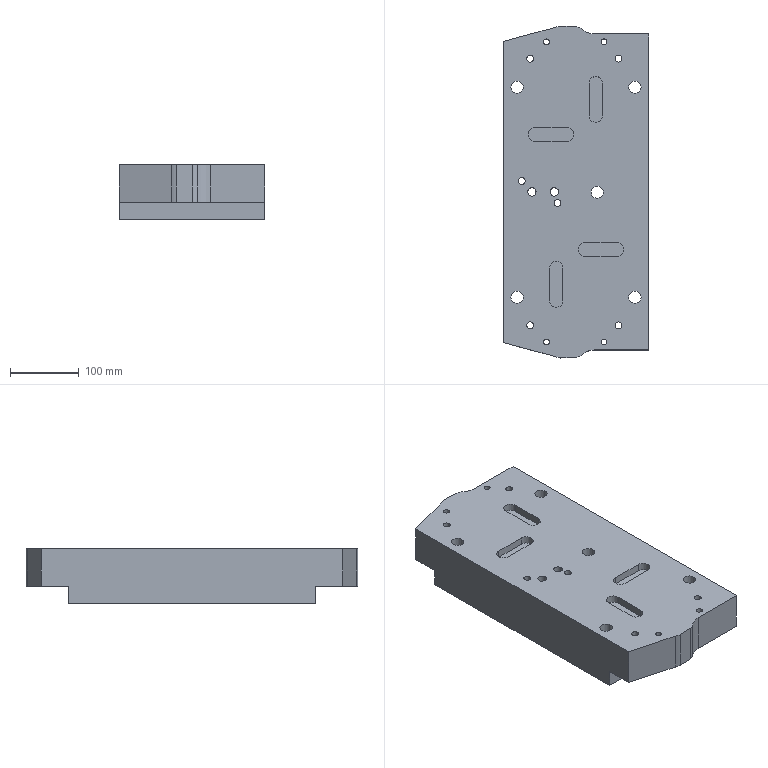Part | STEP file | lll_id650_x_t | 1 solid | 96 faces | box 212 x 484.588 x 80 mm | volume 6932540 mm3 | cylinder 44 | plane 36 | cone 10 | spline 6 | commonest cylinder face diameters 10 x10 8.505 x8 20 x8 18.009 x5 26.007 x5 8.5 x4